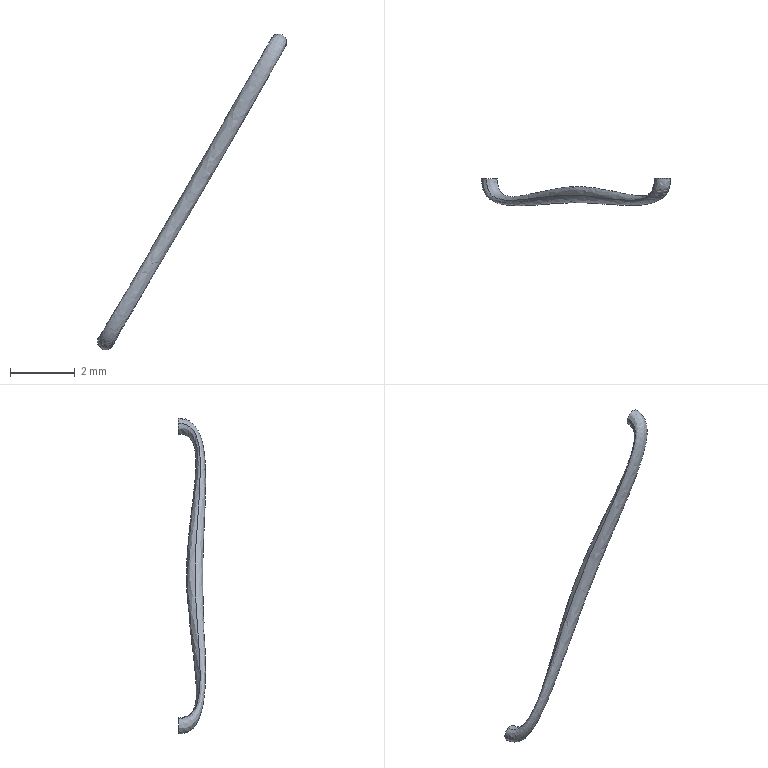Part | SolidWorks | features BaseBody 1 | 1 solid | 4 faces | box 5.839 x 0.8435 x 9.748 mm | volume 1.71 mm3 | plane 2 | spline 2
STEP:
#1=CARTESIAN_POINT('',(328.595,392.451,108.646));
#2=VERTEX_POINT('',#1);
#3=CARTESIAN_POINT('',(328.779,392.451,108.181));
#4=VERTEX_POINT('',#3);
#5=CARTESIAN_POINT('',(328.595,392.451,108.646));
#6=CARTESIAN_POINT('',(328.626,392.451,108.658));
#7=CARTESIAN_POINT('',(328.693,392.451,108.67));
#8=CARTESIAN_POINT('',(328.788,392.451,108.648));
#9=CARTESIAN_POINT('',(328.869,392.451,108.594));
#10=CARTESIAN_POINT('',(328.922,392.452,108.514));
#11=CARTESIAN_POINT('',(328.941,392.452,108.427));
#12=CARTESIAN_POINT('',(328.93,392.452,108.324));
#13=CARTESIAN_POINT('',(328.884,392.452,108.25));
#14=CARTESIAN_POINT('',(328.832,392.451,108.21));
#15=CARTESIAN_POINT('',(328.816,392.451,108.199));
#16=CARTESIAN_POINT('',(328.798,392.451,108.189));
#17=CARTESIAN_POINT('',(328.785,392.451,108.184));
#18=CARTESIAN_POINT('',(328.779,392.451,108.181));
#19=B_SPLINE_CURVE_WITH_KNOTS('',3,(#5,#6,#7,#8,#9,#10,#11,#12,#13,#14,#15,#16,#17,#18),.UNSPECIFIED.,.F.,.F.,(4,1,1,1,1,1,1,1,1,1,1,4),(0.,0.125,0.25,0.375,0.5,0.6,0.7,0.9,0.925,0.95,0.975,1.),.UNSPECIFIED.);
#20=EDGE_CURVE('',#2,#4,#19,.T.);
#21=ORIENTED_EDGE('',*,*,#20,.T.);
#22=CARTESIAN_POINT('',(328.779,392.451,108.181));
#23=CARTESIAN_POINT('',(328.773,392.451,108.179));
#24=CARTESIAN_POINT('',(328.76,392.451,108.174));
#25=CARTESIAN_POINT('',(328.74,392.451,108.169));
#26=CARTESIAN_POINT('',(328.721,392.451,108.166));
#27=CARTESIAN_POINT('',(328.655,392.451,108.159));
#28=CARTESIAN_POINT('',(328.571,392.451,108.182));
#29=CARTESIAN_POINT('',(328.493,392.451,108.249));
#30=CARTESIAN_POINT('',(328.447,392.451,108.326));
#31=CARTESIAN_POINT('',(328.43,392.451,108.42));
#32=CARTESIAN_POINT('',(328.452,392.451,108.515));
#33=CARTESIAN_POINT('',(328.506,392.451,108.596));
#34=CARTESIAN_POINT('',(328.563,392.451,108.634));
#35=CARTESIAN_POINT('',(328.595,392.451,108.646));
#36=B_SPLINE_CURVE_WITH_KNOTS('',3,(#22,#23,#24,#25,#26,#27,#28,#29,#30,#31,#32,#33,#34,#35),.UNSPECIFIED.,.F.,.F.,(4,1,1,1,1,1,1,1,1,1,1,4),(0.,0.025,0.05,0.075,0.1,0.3,0.4,0.5,0.625,0.75,0.875,1.),.UNSPECIFIED.);
#37=EDGE_CURVE('',#4,#2,#36,.T.);
#38=ORIENTED_EDGE('',*,*,#37,.T.);
#39=EDGE_LOOP('',(#21,#38));
#40=FACE_OUTER_BOUND('',#39,.T.);
#41=CARTESIAN_POINT('',(328.687,392.451,108.414));
#42=DIRECTION('',(0.0009599,-1.,0.));
#43=DIRECTION('',(0.,0.,-1.));
#44=AXIS2_PLACEMENT_3D('',#41,#42,#43);
#45=PLANE('',#44);
#46=ADVANCED_FACE('',(#40),#45,.F.);
#47=CARTESIAN_POINT('',(334.259,392.457,117.571));
#48=VERTEX_POINT('',#47);
#49=CARTESIAN_POINT('',(333.793,392.456,117.751));
#50=VERTEX_POINT('',#49);
#51=CARTESIAN_POINT('',(334.259,392.457,117.571));
#52=CARTESIAN_POINT('',(334.256,392.457,117.564));
#53=CARTESIAN_POINT('',(334.251,392.457,117.552));
#54=CARTESIAN_POINT('',(334.241,392.457,117.534));
#55=CARTESIAN_POINT('',(334.231,392.457,117.517));
#56=CARTESIAN_POINT('',(334.191,392.457,117.465));
#57=CARTESIAN_POINT('',(334.117,392.457,117.419));
#58=CARTESIAN_POINT('',(334.014,392.456,117.407));
#59=CARTESIAN_POINT('',(333.927,392.456,117.425));
#60=CARTESIAN_POINT('',(333.847,392.456,117.477));
#61=CARTESIAN_POINT('',(333.792,392.456,117.558));
#62=CARTESIAN_POINT('',(333.769,392.456,117.653));
#63=CARTESIAN_POINT('',(333.781,392.456,117.72));
#64=CARTESIAN_POINT('',(333.793,392.456,117.751));
#65=B_SPLINE_CURVE_WITH_KNOTS('',3,(#51,#52,#53,#54,#55,#56,#57,#58,#59,#60,#61,#62,#63,#64),.UNSPECIFIED.,.F.,.F.,(4,1,1,1,1,1,1,1,1,1,1,4),(0.,0.025,0.05,0.075,0.1,0.3,0.4,0.5,0.625,0.75,0.875,1.),.UNSPECIFIED.);
#66=EDGE_CURVE('',#48,#50,#65,.T.);
#67=ORIENTED_EDGE('',*,*,#66,.T.);
#68=CARTESIAN_POINT('',(333.793,392.456,117.751));
#69=CARTESIAN_POINT('',(333.805,392.456,117.783));
#70=CARTESIAN_POINT('',(333.842,392.456,117.84));
#71=CARTESIAN_POINT('',(333.923,392.456,117.895));
#72=CARTESIAN_POINT('',(334.017,392.456,117.917));
#73=CARTESIAN_POINT('',(334.112,392.457,117.902));
#74=CARTESIAN_POINT('',(334.189,392.457,117.856));
#75=CARTESIAN_POINT('',(334.257,392.457,117.778));
#76=CARTESIAN_POINT('',(334.28,392.457,117.695));
#77=CARTESIAN_POINT('',(334.274,392.457,117.629));
#78=CARTESIAN_POINT('',(334.271,392.457,117.609));
#79=CARTESIAN_POINT('',(334.266,392.457,117.59));
#80=CARTESIAN_POINT('',(334.261,392.457,117.577));
#81=CARTESIAN_POINT('',(334.259,392.457,117.571));
#82=B_SPLINE_CURVE_WITH_KNOTS('',3,(#68,#69,#70,#71,#72,#73,#74,#75,#76,#77,#78,#79,#80,#81),.UNSPECIFIED.,.F.,.F.,(4,1,1,1,1,1,1,1,1,1,1,4),(0.,0.125,0.25,0.375,0.5,0.6,0.7,0.9,0.925,0.95,0.975,1.),.UNSPECIFIED.);
#83=EDGE_CURVE('',#50,#48,#82,.T.);
#84=ORIENTED_EDGE('',*,*,#83,.T.);
#85=EDGE_LOOP('',(#67,#84));
#86=FACE_OUTER_BOUND('',#85,.T.);
#87=CARTESIAN_POINT('',(334.026,392.456,117.661));
#88=DIRECTION('',(0.0009599,-1.,0.));
#89=DIRECTION('',(0.,0.,-1.));
#90=AXIS2_PLACEMENT_3D('',#87,#88,#89);
#91=PLANE('',#90);
#92=ADVANCED_FACE('',(#86),#91,.F.);
#93=CARTESIAN_POINT('',(328.595,392.451,108.646));
#94=CARTESIAN_POINT('',(328.596,391.341,108.646));
#95=CARTESIAN_POINT('',(331.131,392.551,113.099));
#96=CARTESIAN_POINT('',(333.794,391.323,117.751));
#97=CARTESIAN_POINT('',(333.793,392.456,117.751));
#98=B_SPLINE_CURVE_WITH_KNOTS('',3,(#93,#94,#95,#96,#97),.UNSPECIFIED.,.F.,.F.,(4,1,4),(0.,0.5,1.),.UNSPECIFIED.);
#99=EDGE_CURVE('',#2,#50,#98,.T.);
#100=ORIENTED_EDGE('',*,*,#99,.F.);
#101=ORIENTED_EDGE('',*,*,#37,.F.);
#102=CARTESIAN_POINT('',(334.259,392.457,117.571));
#103=CARTESIAN_POINT('',(334.26,391.312,117.571));
#104=CARTESIAN_POINT('',(331.671,392.636,112.923));
#105=CARTESIAN_POINT('',(328.78,391.283,108.181));
#106=CARTESIAN_POINT('',(328.779,392.451,108.181));
#107=B_SPLINE_CURVE_WITH_KNOTS('',3,(#102,#103,#104,#105,#106),.UNSPECIFIED.,.F.,.F.,(4,1,4),(0.,0.5,1.),.UNSPECIFIED.);
#108=EDGE_CURVE('',#48,#4,#107,.T.);
#109=ORIENTED_EDGE('',*,*,#108,.F.);
#110=ORIENTED_EDGE('',*,*,#83,.F.);
#111=EDGE_LOOP('',(#100,#101,#109,#110));
#112=FACE_OUTER_BOUND('',#111,.T.);
#113=CARTESIAN_POINT('',(334.249,392.568,117.549));
#114=CARTESIAN_POINT('',(334.334,391.275,117.699));
#115=CARTESIAN_POINT('',(331.665,392.707,112.922));
#116=CARTESIAN_POINT('',(328.696,391.24,108.025));
#117=CARTESIAN_POINT('',(328.798,392.577,108.196));
#118=CARTESIAN_POINT('',(334.251,392.568,117.554));
#119=CARTESIAN_POINT('',(334.336,391.273,117.704));
#120=CARTESIAN_POINT('',(331.667,392.698,112.92));
#121=CARTESIAN_POINT('',(328.691,391.239,108.023));
#122=CARTESIAN_POINT('',(328.794,392.578,108.194));
#123=CARTESIAN_POINT('',(334.256,392.568,117.565));
#124=CARTESIAN_POINT('',(334.341,391.27,117.716));
#125=CARTESIAN_POINT('',(331.672,392.677,112.916));
#126=CARTESIAN_POINT('',(328.68,391.236,108.018));
#127=CARTESIAN_POINT('',(328.783,392.578,108.189));
#128=CARTESIAN_POINT('',(334.262,392.569,117.583));
#129=CARTESIAN_POINT('',(334.347,391.264,117.735));
#130=CARTESIAN_POINT('',(331.679,392.645,112.91));
#131=CARTESIAN_POINT('',(328.661,391.231,108.012));
#132=CARTESIAN_POINT('',(328.765,392.578,108.183));
#133=CARTESIAN_POINT('',(334.267,392.57,117.603));
#134=CARTESIAN_POINT('',(334.352,391.258,117.755));
#135=CARTESIAN_POINT('',(331.684,392.61,112.903));
#136=CARTESIAN_POINT('',(328.641,391.226,108.007));
#137=CARTESIAN_POINT('',(328.745,392.579,108.177));
#138=CARTESIAN_POINT('',(334.27,392.57,117.622));
#139=CARTESIAN_POINT('',(334.355,391.252,117.775));
#140=CARTESIAN_POINT('',(331.687,392.576,112.898));
#141=CARTESIAN_POINT('',(328.62,391.221,108.003));
#142=CARTESIAN_POINT('',(328.726,392.58,108.174));
#143=CARTESIAN_POINT('',(334.276,392.572,117.688));
#144=CARTESIAN_POINT('',(334.361,391.233,117.843));
#145=CARTESIAN_POINT('',(331.692,392.464,112.882));
#146=CARTESIAN_POINT('',(328.552,391.207,107.997));
#147=CARTESIAN_POINT('',(328.66,392.581,108.168));
#148=CARTESIAN_POINT('',(334.253,392.574,117.771));
#149=CARTESIAN_POINT('',(334.338,391.212,117.93));
#150=CARTESIAN_POINT('',(331.663,392.337,112.875));
#151=CARTESIAN_POINT('',(328.467,391.194,108.021));
#152=CARTESIAN_POINT('',(328.577,392.583,108.19));
#153=CARTESIAN_POINT('',(334.185,392.575,117.849));
#154=CARTESIAN_POINT('',(334.27,391.2,118.01));
#155=CARTESIAN_POINT('',(331.581,392.238,112.89));
#156=CARTESIAN_POINT('',(328.388,391.193,108.09));
#157=CARTESIAN_POINT('',(328.498,392.583,108.258));
#158=CARTESIAN_POINT('',(334.108,392.576,117.895));
#159=CARTESIAN_POINT('',(334.194,391.198,118.056));
#160=CARTESIAN_POINT('',(331.491,392.198,112.915));
#161=CARTESIAN_POINT('',(328.344,391.2,108.168));
#162=CARTESIAN_POINT('',(328.452,392.582,108.334));
#163=CARTESIAN_POINT('',(334.013,392.575,117.91));
#164=CARTESIAN_POINT('',(334.1,391.208,118.071));
#165=CARTESIAN_POINT('',(331.381,392.214,112.954));
#166=CARTESIAN_POINT('',(328.33,391.217,108.264));
#167=CARTESIAN_POINT('',(328.435,392.58,108.428));
#168=CARTESIAN_POINT('',(333.919,392.572,117.888));
#169=CARTESIAN_POINT('',(334.006,391.229,118.046));
#170=CARTESIAN_POINT('',(331.271,392.292,113.001));
#171=CARTESIAN_POINT('',(328.356,391.244,108.361));
#172=CARTESIAN_POINT('',(328.457,392.577,108.523));
#173=CARTESIAN_POINT('',(333.838,392.57,117.833));
#174=CARTESIAN_POINT('',(333.926,391.256,117.988));
#175=CARTESIAN_POINT('',(331.18,392.418,113.048));
#176=CARTESIAN_POINT('',(328.416,391.273,108.443));
#177=CARTESIAN_POINT('',(328.511,392.574,108.604));
#178=CARTESIAN_POINT('',(333.798,392.567,117.772));
#179=CARTESIAN_POINT('',(333.886,391.276,117.924));
#180=CARTESIAN_POINT('',(331.135,392.541,113.079));
#181=CARTESIAN_POINT('',(328.481,391.292,108.484));
#182=CARTESIAN_POINT('',(328.572,392.572,108.644));
#183=CARTESIAN_POINT('',(333.785,392.566,117.735));
#184=CARTESIAN_POINT('',(333.873,391.287,117.886));
#185=CARTESIAN_POINT('',(331.121,392.609,113.092));
#186=CARTESIAN_POINT('',(328.519,391.301,108.497));
#187=CARTESIAN_POINT('',(328.608,392.571,108.657));
#188=CARTESIAN_POINT('',(333.784,392.566,117.73));
#189=CARTESIAN_POINT('',(333.871,391.288,117.88));
#190=CARTESIAN_POINT('',(331.119,392.618,113.094));
#191=CARTESIAN_POINT('',(328.524,391.302,108.499));
#192=CARTESIAN_POINT('',(328.613,392.571,108.659));
#193=B_SPLINE_SURFACE_WITH_KNOTS('',3,3,((#113,#114,#115,#116,#117),(#118,#119,#120,#121,#122),(#123,#124,#125,#126,#127),(#128,#129,#130,#131,#132),(#133,#134,#135,#136,#137),(#138,#139,#140,#141,#142),(#143,#144,#145,#146,#147),(#148,#149,#150,#151,#152),(#153,#154,#155,#156,#157),(#158,#159,#160,#161,#162),(#163,#164,#165,#166,#167),(#168,#169,#170,#171,#172),(#173,#174,#175,#176,#177),(#178,#179,#180,#181,#182),(#183,#184,#185,#186,#187),(#188,#189,#190,#191,#192)),.UNSPECIFIED.,.F.,.F.,.F.,(4,1,1,1,1,1,1,1,1,1,1,1,1,4),(4,1,4),(-0.009538,0.,0.0125,0.025,0.0375,0.05,0.15,0.2,0.25,0.3125,0.375,0.4375,0.5,0.5095),(-0.01548,0.5,1.017),.UNSPECIFIED.);
#194=ADVANCED_FACE('',(#112),#193,.T.);
#195=ORIENTED_EDGE('',*,*,#66,.F.);
#196=ORIENTED_EDGE('',*,*,#108,.T.);
#197=ORIENTED_EDGE('',*,*,#20,.F.);
#198=ORIENTED_EDGE('',*,*,#99,.T.);
#199=EDGE_LOOP('',(#195,#196,#197,#198));
#200=FACE_OUTER_BOUND('',#199,.T.);
#201=CARTESIAN_POINT('',(333.795,392.567,117.759));
#202=CARTESIAN_POINT('',(333.882,391.28,117.91));
#203=CARTESIAN_POINT('',(331.132,392.564,113.083));
#204=CARTESIAN_POINT('',(328.494,391.295,108.487));
#205=CARTESIAN_POINT('',(328.585,392.572,108.648));
#206=CARTESIAN_POINT('',(333.793,392.567,117.754));
#207=CARTESIAN_POINT('',(333.88,391.281,117.905));
#208=CARTESIAN_POINT('',(331.129,392.573,113.085));
#209=CARTESIAN_POINT('',(328.499,391.297,108.49));
#210=CARTESIAN_POINT('',(328.589,392.572,108.65));
#211=CARTESIAN_POINT('',(333.778,392.566,117.719));
#212=CARTESIAN_POINT('',(333.865,391.292,117.868));
#213=CARTESIAN_POINT('',(331.113,392.64,113.099));
#214=CARTESIAN_POINT('',(328.536,391.306,108.505));
#215=CARTESIAN_POINT('',(328.625,392.571,108.665));
#216=CARTESIAN_POINT('',(333.765,392.564,117.646));
#217=CARTESIAN_POINT('',(333.853,391.311,117.793));
#218=CARTESIAN_POINT('',(331.101,392.769,113.119));
#219=CARTESIAN_POINT('',(328.612,391.32,108.518));
#220=CARTESIAN_POINT('',(328.697,392.569,108.678));
#221=CARTESIAN_POINT('',(333.788,392.561,117.551));
#222=CARTESIAN_POINT('',(333.875,391.334,117.695));
#223=CARTESIAN_POINT('',(331.129,392.917,113.129));
#224=CARTESIAN_POINT('',(328.709,391.334,108.495));
#225=CARTESIAN_POINT('',(328.792,392.567,108.656));
#226=CARTESIAN_POINT('',(333.843,392.56,117.471));
#227=CARTESIAN_POINT('',(333.93,391.35,117.612));
#228=CARTESIAN_POINT('',(331.196,393.025,113.12));
#229=CARTESIAN_POINT('',(328.79,391.339,108.439));
#230=CARTESIAN_POINT('',(328.873,392.567,108.602));
#231=CARTESIAN_POINT('',(333.923,392.559,117.419));
#232=CARTESIAN_POINT('',(334.009,391.355,117.559));
#233=CARTESIAN_POINT('',(331.29,393.073,113.095));
#234=CARTESIAN_POINT('',(328.842,391.334,108.357));
#235=CARTESIAN_POINT('',(328.926,392.567,108.522));
#236=CARTESIAN_POINT('',(334.01,392.56,117.401));
#237=CARTESIAN_POINT('',(334.096,391.348,117.541));
#238=CARTESIAN_POINT('',(331.392,393.063,113.06));
#239=CARTESIAN_POINT('',(328.858,391.32,108.269));
#240=CARTESIAN_POINT('',(328.945,392.569,108.435));
#241=CARTESIAN_POINT('',(334.113,392.562,117.412));
#242=CARTESIAN_POINT('',(334.199,391.331,117.555));
#243=CARTESIAN_POINT('',(331.512,392.997,113.011));
#244=CARTESIAN_POINT('',(328.842,391.296,108.163));
#245=CARTESIAN_POINT('',(328.934,392.571,108.332));
#246=CARTESIAN_POINT('',(334.187,392.564,117.458));
#247=CARTESIAN_POINT('',(334.272,391.308,117.604));
#248=CARTESIAN_POINT('',(331.595,392.887,112.969));
#249=CARTESIAN_POINT('',(328.793,391.271,108.089));
#250=CARTESIAN_POINT('',(328.889,392.574,108.259));
#251=CARTESIAN_POINT('',(334.227,392.566,117.51));
#252=CARTESIAN_POINT('',(334.312,391.289,117.659));
#253=CARTESIAN_POINT('',(331.64,392.782,112.94));
#254=CARTESIAN_POINT('',(328.737,391.253,108.048));
#255=CARTESIAN_POINT('',(328.837,392.576,108.218));
#256=CARTESIAN_POINT('',(334.238,392.567,117.527));
#257=CARTESIAN_POINT('',(334.323,391.283,117.676));
#258=CARTESIAN_POINT('',(331.652,392.749,112.932));
#259=CARTESIAN_POINT('',(328.72,391.247,108.037));
#260=CARTESIAN_POINT('',(328.821,392.577,108.207));
#261=CARTESIAN_POINT('',(334.247,392.568,117.545));
#262=CARTESIAN_POINT('',(334.332,391.276,117.695));
#263=CARTESIAN_POINT('',(331.663,392.715,112.924));
#264=CARTESIAN_POINT('',(328.701,391.242,108.027));
#265=CARTESIAN_POINT('',(328.803,392.577,108.198));
#266=CARTESIAN_POINT('',(334.255,392.568,117.562));
#267=CARTESIAN_POINT('',(334.34,391.271,117.713));
#268=CARTESIAN_POINT('',(331.671,392.683,112.917));
#269=CARTESIAN_POINT('',(328.683,391.236,108.019));
#270=CARTESIAN_POINT('',(328.786,392.578,108.19));
#271=CARTESIAN_POINT('',(334.259,392.569,117.574));
#272=CARTESIAN_POINT('',(334.344,391.267,117.725));
#273=CARTESIAN_POINT('',(331.675,392.662,112.913));
#274=CARTESIAN_POINT('',(328.671,391.233,108.015));
#275=CARTESIAN_POINT('',(328.774,392.578,108.186));
#276=CARTESIAN_POINT('',(334.26,392.569,117.579));
#277=CARTESIAN_POINT('',(334.345,391.265,117.73));
#278=CARTESIAN_POINT('',(331.677,392.653,112.911));
#279=CARTESIAN_POINT('',(328.666,391.232,108.014));
#280=CARTESIAN_POINT('',(328.769,392.578,108.184));
#281=B_SPLINE_SURFACE_WITH_KNOTS('',3,3,((#201,#202,#203,#204,#205),(#206,#207,#208,#209,#210),(#211,#212,#213,#214,#215),(#216,#217,#218,#219,#220),(#221,#222,#223,#224,#225),(#226,#227,#228,#229,#230),(#231,#232,#233,#234,#235),(#236,#237,#238,#239,#240),(#241,#242,#243,#244,#245),(#246,#247,#248,#249,#250),(#251,#252,#253,#254,#255),(#256,#257,#258,#259,#260),(#261,#262,#263,#264,#265),(#266,#267,#268,#269,#270),(#271,#272,#273,#274,#275),(#276,#277,#278,#279,#280)),.UNSPECIFIED.,.F.,.F.,.F.,(4,1,1,1,1,1,1,1,1,1,1,1,1,4),(4,1,4),(0.4905,0.5,0.5625,0.625,0.6875,0.75,0.8,0.85,0.95,0.9625,0.975,0.9875,1.,1.01),(-0.01548,0.5,1.017),.UNSPECIFIED.);
#282=ADVANCED_FACE('',(#200),#281,.T.);
#283=CLOSED_SHELL('',(#46,#92,#194,#282));
#284=MANIFOLD_SOLID_BREP('',#283);
#285=CARTESIAN_POINT('',(0.,0.,0.));
#286=DIRECTION('',(0.,0.,1.));
#287=DIRECTION('',(1.,0.,0.));
#288=AXIS2_PLACEMENT_3D('',#285,#286,#287);
#289=(LENGTH_UNIT()NAMED_UNIT(*)SI_UNIT(.MILLI.,.METRE.));
#290=UNCERTAINTY_MEASURE_WITH_UNIT(LENGTH_MEASURE(0.00001),#289,'','');
#291=(NAMED_UNIT(*)PLANE_ANGLE_UNIT()SI_UNIT($,.RADIAN.));
#292=(NAMED_UNIT(*)SI_UNIT($,.STERADIAN.)SOLID_ANGLE_UNIT());
#293=(GEOMETRIC_REPRESENTATION_CONTEXT(3)GLOBAL_UNCERTAINTY_ASSIGNED_CONTEXT((#290))GLOBAL_UNIT_ASSIGNED_CONTEXT((#289,#291,#292))REPRESENTATION_CONTEXT('',''));
#294=ADVANCED_BREP_SHAPE_REPRESENTATION('',(#284,#288),#293);